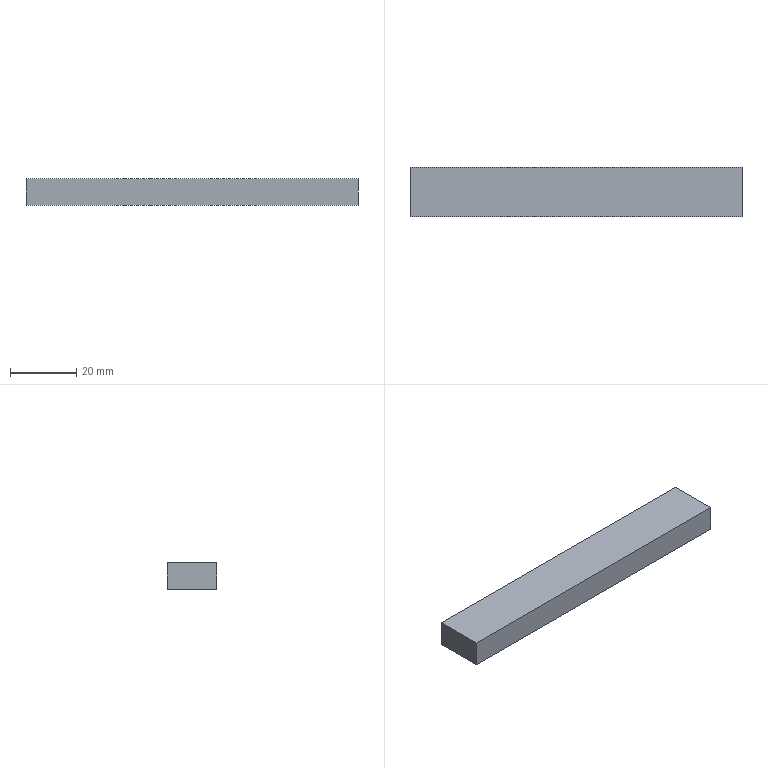Part | SolidWorks | features Extrusion 1 | 1 solid | 6 faces | box 100 x 15 x 8 mm | volume 12000 mm3 | plane 6
STEP:
#1=CARTESIAN_POINT('',(50.,-7.5,0.));
#2=VERTEX_POINT('',#1);
#3=CARTESIAN_POINT('',(50.,7.5,0.));
#4=VERTEX_POINT('',#3);
#5=CARTESIAN_POINT('',(50.,-7.5,0.));
#6=DIRECTION('',(0.,1.,0.));
#7=VECTOR('',#6,1000.);
#8=LINE('',#5,#7);
#9=EDGE_CURVE('',#2,#4,#8,.T.);
#10=ORIENTED_EDGE('',*,*,#9,.T.);
#11=CARTESIAN_POINT('',(50.,7.5,8.));
#12=VERTEX_POINT('',#11);
#13=CARTESIAN_POINT('',(50.,7.5,8.));
#14=DIRECTION('',(0.,0.,-1.));
#15=VECTOR('',#14,1000.);
#16=LINE('',#13,#15);
#17=EDGE_CURVE('',#12,#4,#16,.T.);
#18=ORIENTED_EDGE('',*,*,#17,.F.);
#19=CARTESIAN_POINT('',(50.,-7.5,8.));
#20=VERTEX_POINT('',#19);
#21=CARTESIAN_POINT('',(50.,-7.5,8.));
#22=DIRECTION('',(0.,1.,0.));
#23=VECTOR('',#22,1000.);
#24=LINE('',#21,#23);
#25=EDGE_CURVE('',#20,#12,#24,.T.);
#26=ORIENTED_EDGE('',*,*,#25,.F.);
#27=CARTESIAN_POINT('',(50.,-7.5,8.));
#28=DIRECTION('',(0.,0.,-1.));
#29=VECTOR('',#28,1000.);
#30=LINE('',#27,#29);
#31=EDGE_CURVE('',#20,#2,#30,.T.);
#32=ORIENTED_EDGE('',*,*,#31,.T.);
#33=EDGE_LOOP('',(#10,#18,#26,#32));
#34=FACE_OUTER_BOUND('',#33,.T.);
#35=CARTESIAN_POINT('',(50.,-7.5,8.));
#36=DIRECTION('',(-1.,0.,0.));
#37=DIRECTION('',(0.,0.,1.));
#38=AXIS2_PLACEMENT_3D('',#35,#36,#37);
#39=PLANE('',#38);
#40=ADVANCED_FACE('',(#34),#39,.F.);
#41=CARTESIAN_POINT('',(-50.,7.5,0.));
#42=VERTEX_POINT('',#41);
#43=CARTESIAN_POINT('',(-50.,7.5,0.));
#44=DIRECTION('',(-1.,0.,0.));
#45=VECTOR('',#44,1000.);
#46=LINE('',#43,#45);
#47=EDGE_CURVE('',#4,#42,#46,.T.);
#48=ORIENTED_EDGE('',*,*,#47,.T.);
#49=CARTESIAN_POINT('',(-50.,7.5,8.));
#50=VERTEX_POINT('',#49);
#51=CARTESIAN_POINT('',(-50.,7.5,8.));
#52=DIRECTION('',(0.,0.,-1.));
#53=VECTOR('',#52,1000.);
#54=LINE('',#51,#53);
#55=EDGE_CURVE('',#50,#42,#54,.T.);
#56=ORIENTED_EDGE('',*,*,#55,.F.);
#57=CARTESIAN_POINT('',(-50.,7.5,8.));
#58=DIRECTION('',(-1.,0.,0.));
#59=VECTOR('',#58,1000.);
#60=LINE('',#57,#59);
#61=EDGE_CURVE('',#12,#50,#60,.T.);
#62=ORIENTED_EDGE('',*,*,#61,.F.);
#63=ORIENTED_EDGE('',*,*,#17,.T.);
#64=EDGE_LOOP('',(#48,#56,#62,#63));
#65=FACE_OUTER_BOUND('',#64,.T.);
#66=CARTESIAN_POINT('',(-50.,7.5,8.));
#67=DIRECTION('',(0.,-1.,0.));
#68=DIRECTION('',(0.,0.,-1.));
#69=AXIS2_PLACEMENT_3D('',#66,#67,#68);
#70=PLANE('',#69);
#71=ADVANCED_FACE('',(#65),#70,.F.);
#72=CARTESIAN_POINT('',(-50.,-7.5,0.));
#73=VERTEX_POINT('',#72);
#74=CARTESIAN_POINT('',(-50.,-7.5,0.));
#75=DIRECTION('',(0.,-1.,0.));
#76=VECTOR('',#75,1000.);
#77=LINE('',#74,#76);
#78=EDGE_CURVE('',#42,#73,#77,.T.);
#79=ORIENTED_EDGE('',*,*,#78,.T.);
#80=CARTESIAN_POINT('',(-50.,-7.5,8.));
#81=VERTEX_POINT('',#80);
#82=CARTESIAN_POINT('',(-50.,-7.5,8.));
#83=DIRECTION('',(0.,0.,-1.));
#84=VECTOR('',#83,1000.);
#85=LINE('',#82,#84);
#86=EDGE_CURVE('',#81,#73,#85,.T.);
#87=ORIENTED_EDGE('',*,*,#86,.F.);
#88=CARTESIAN_POINT('',(-50.,-7.5,8.));
#89=DIRECTION('',(0.,-1.,0.));
#90=VECTOR('',#89,1000.);
#91=LINE('',#88,#90);
#92=EDGE_CURVE('',#50,#81,#91,.T.);
#93=ORIENTED_EDGE('',*,*,#92,.F.);
#94=ORIENTED_EDGE('',*,*,#55,.T.);
#95=EDGE_LOOP('',(#79,#87,#93,#94));
#96=FACE_OUTER_BOUND('',#95,.T.);
#97=CARTESIAN_POINT('',(-50.,-7.5,8.));
#98=DIRECTION('',(1.,0.,0.));
#99=DIRECTION('',(0.,0.,-1.));
#100=AXIS2_PLACEMENT_3D('',#97,#98,#99);
#101=PLANE('',#100);
#102=ADVANCED_FACE('',(#96),#101,.F.);
#103=CARTESIAN_POINT('',(-50.,-7.5,0.));
#104=DIRECTION('',(1.,0.,0.));
#105=VECTOR('',#104,1000.);
#106=LINE('',#103,#105);
#107=EDGE_CURVE('',#73,#2,#106,.T.);
#108=ORIENTED_EDGE('',*,*,#107,.T.);
#109=ORIENTED_EDGE('',*,*,#31,.F.);
#110=CARTESIAN_POINT('',(-50.,-7.5,8.));
#111=DIRECTION('',(1.,0.,0.));
#112=VECTOR('',#111,1000.);
#113=LINE('',#110,#112);
#114=EDGE_CURVE('',#81,#20,#113,.T.);
#115=ORIENTED_EDGE('',*,*,#114,.F.);
#116=ORIENTED_EDGE('',*,*,#86,.T.);
#117=EDGE_LOOP('',(#108,#109,#115,#116));
#118=FACE_OUTER_BOUND('',#117,.T.);
#119=CARTESIAN_POINT('',(-50.,-7.5,8.));
#120=DIRECTION('',(0.,1.,0.));
#121=DIRECTION('',(0.,0.,1.));
#122=AXIS2_PLACEMENT_3D('',#119,#120,#121);
#123=PLANE('',#122);
#124=ADVANCED_FACE('',(#118),#123,.F.);
#125=ORIENTED_EDGE('',*,*,#25,.T.);
#126=ORIENTED_EDGE('',*,*,#61,.T.);
#127=ORIENTED_EDGE('',*,*,#92,.T.);
#128=ORIENTED_EDGE('',*,*,#114,.T.);
#129=EDGE_LOOP('',(#125,#126,#127,#128));
#130=FACE_OUTER_BOUND('',#129,.T.);
#131=CARTESIAN_POINT('',(0.,0.,8.));
#132=DIRECTION('',(0.,0.,-1.));
#133=DIRECTION('',(-1.,0.,0.));
#134=AXIS2_PLACEMENT_3D('',#131,#132,#133);
#135=PLANE('',#134);
#136=ADVANCED_FACE('',(#130),#135,.F.);
#137=ORIENTED_EDGE('',*,*,#9,.F.);
#138=ORIENTED_EDGE('',*,*,#107,.F.);
#139=ORIENTED_EDGE('',*,*,#78,.F.);
#140=ORIENTED_EDGE('',*,*,#47,.F.);
#141=EDGE_LOOP('',(#137,#138,#139,#140));
#142=FACE_OUTER_BOUND('',#141,.T.);
#143=CARTESIAN_POINT('',(0.,0.,0.));
#144=DIRECTION('',(0.,0.,-1.));
#145=DIRECTION('',(-1.,0.,0.));
#146=AXIS2_PLACEMENT_3D('',#143,#144,#145);
#147=PLANE('',#146);
#148=ADVANCED_FACE('',(#142),#147,.T.);
#149=CLOSED_SHELL('',(#40,#71,#102,#124,#136,#148));
#150=MANIFOLD_SOLID_BREP('',#149);
#151=CARTESIAN_POINT('',(0.,0.,0.));
#152=DIRECTION('',(0.,0.,1.));
#153=DIRECTION('',(1.,0.,0.));
#154=AXIS2_PLACEMENT_3D('',#151,#152,#153);
#155=(LENGTH_UNIT()NAMED_UNIT(*)SI_UNIT(.MILLI.,.METRE.));
#156=UNCERTAINTY_MEASURE_WITH_UNIT(LENGTH_MEASURE(0.00001),#155,'','');
#157=(NAMED_UNIT(*)PLANE_ANGLE_UNIT()SI_UNIT($,.RADIAN.));
#158=(NAMED_UNIT(*)SI_UNIT($,.STERADIAN.)SOLID_ANGLE_UNIT());
#159=(GEOMETRIC_REPRESENTATION_CONTEXT(3)GLOBAL_UNCERTAINTY_ASSIGNED_CONTEXT((#156))GLOBAL_UNIT_ASSIGNED_CONTEXT((#155,#157,#158))REPRESENTATION_CONTEXT('',''));
#160=ADVANCED_BREP_SHAPE_REPRESENTATION('',(#150,#154),#159);